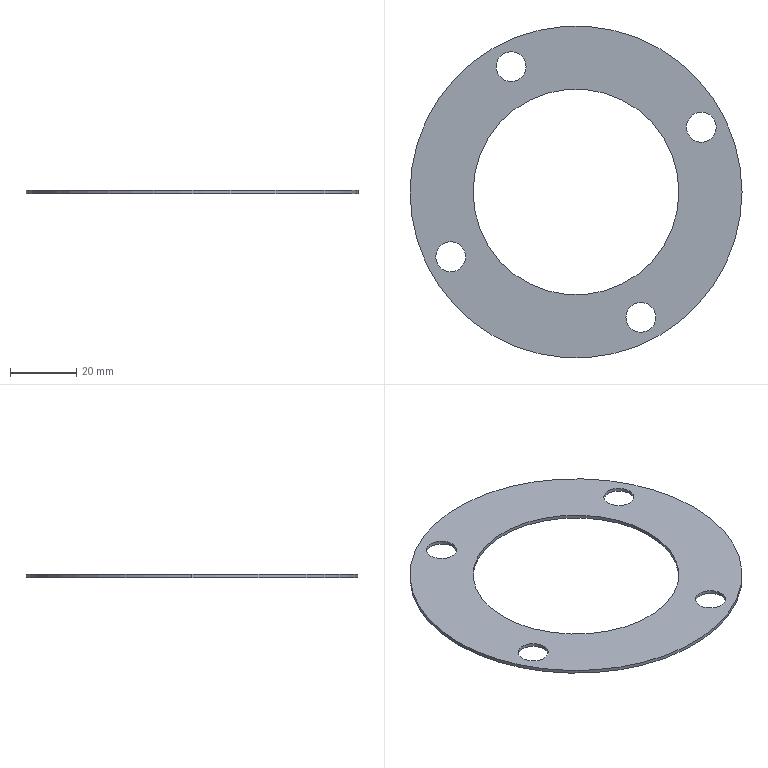Part | SolidWorks | features BaseBody 1 | 1 solid | 14 faces | box 100 x 100 x 1 mm | volume 4580 mm3 | cylinder 12 | plane 2 | commonest cylinder face diameters 9 x8 62 x2 100 x2
STEP:
#1=CARTESIAN_POINT('',(41.434,-38.434,0.));
#2=VERTEX_POINT('',#1);
#3=CARTESIAN_POINT('',(50.434,-38.434,0.));
#4=VERTEX_POINT('',#3);
#5=CARTESIAN_POINT('',(45.934,-38.434,0.));
#6=DIRECTION('',(0.,0.,1.));
#7=DIRECTION('',(1.,0.,0.));
#8=AXIS2_PLACEMENT_3D('',#5,#6,#7);
#9=CIRCLE('',#8,4.5);
#10=EDGE_CURVE('',#2,#4,#9,.T.);
#11=ORIENTED_EDGE('',*,*,#10,.F.);
#12=CARTESIAN_POINT('',(41.434,-38.434,1.));
#13=VERTEX_POINT('',#12);
#14=CARTESIAN_POINT('',(41.434,-38.434,0.));
#15=DIRECTION('',(0.,0.,1.));
#16=VECTOR('',#15,1000.);
#17=LINE('',#14,#16);
#18=EDGE_CURVE('',#2,#13,#17,.T.);
#19=ORIENTED_EDGE('',*,*,#18,.T.);
#20=CARTESIAN_POINT('',(50.434,-38.434,1.));
#21=VERTEX_POINT('',#20);
#22=CARTESIAN_POINT('',(45.934,-38.434,1.));
#23=DIRECTION('',(0.,0.,-1.));
#24=DIRECTION('',(1.,0.,0.));
#25=AXIS2_PLACEMENT_3D('',#22,#23,#24);
#26=CIRCLE('',#25,4.5);
#27=EDGE_CURVE('',#21,#13,#26,.T.);
#28=ORIENTED_EDGE('',*,*,#27,.F.);
#29=CARTESIAN_POINT('',(50.434,-38.434,0.));
#30=DIRECTION('',(0.,0.,1.));
#31=VECTOR('',#30,1000.);
#32=LINE('',#29,#31);
#33=EDGE_CURVE('',#4,#21,#32,.T.);
#34=ORIENTED_EDGE('',*,*,#33,.F.);
#35=EDGE_LOOP('',(#11,#19,#28,#34));
#36=FACE_OUTER_BOUND('',#35,.T.);
#37=CARTESIAN_POINT('',(45.934,-38.434,0.));
#38=DIRECTION('',(0.,0.,1.));
#39=DIRECTION('',(1.,0.,0.));
#40=AXIS2_PLACEMENT_3D('',#37,#38,#39);
#41=CYLINDRICAL_SURFACE('',#40,4.5);
#42=ADVANCED_FACE('',(#36),#41,.F.);
#43=CARTESIAN_POINT('',(59.662,18.839,0.));
#44=VERTEX_POINT('',#43);
#45=CARTESIAN_POINT('',(68.662,18.839,0.));
#46=VERTEX_POINT('',#45);
#47=CARTESIAN_POINT('',(64.162,18.839,0.));
#48=DIRECTION('',(0.,0.,1.));
#49=DIRECTION('',(1.,0.,0.));
#50=AXIS2_PLACEMENT_3D('',#47,#48,#49);
#51=CIRCLE('',#50,4.5);
#52=EDGE_CURVE('',#44,#46,#51,.T.);
#53=ORIENTED_EDGE('',*,*,#52,.F.);
#54=CARTESIAN_POINT('',(59.662,18.839,1.));
#55=VERTEX_POINT('',#54);
#56=CARTESIAN_POINT('',(59.662,18.839,0.));
#57=DIRECTION('',(0.,0.,1.));
#58=VECTOR('',#57,1000.);
#59=LINE('',#56,#58);
#60=EDGE_CURVE('',#44,#55,#59,.T.);
#61=ORIENTED_EDGE('',*,*,#60,.T.);
#62=CARTESIAN_POINT('',(68.662,18.839,1.));
#63=VERTEX_POINT('',#62);
#64=CARTESIAN_POINT('',(64.162,18.839,1.));
#65=DIRECTION('',(0.,0.,-1.));
#66=DIRECTION('',(1.,0.,0.));
#67=AXIS2_PLACEMENT_3D('',#64,#65,#66);
#68=CIRCLE('',#67,4.5);
#69=EDGE_CURVE('',#63,#55,#68,.T.);
#70=ORIENTED_EDGE('',*,*,#69,.F.);
#71=CARTESIAN_POINT('',(68.662,18.839,0.));
#72=DIRECTION('',(0.,0.,1.));
#73=VECTOR('',#72,1000.);
#74=LINE('',#71,#73);
#75=EDGE_CURVE('',#46,#63,#74,.T.);
#76=ORIENTED_EDGE('',*,*,#75,.F.);
#77=EDGE_LOOP('',(#53,#61,#70,#76));
#78=FACE_OUTER_BOUND('',#77,.T.);
#79=CARTESIAN_POINT('',(64.162,18.839,0.));
#80=DIRECTION('',(0.,0.,1.));
#81=DIRECTION('',(1.,0.,0.));
#82=AXIS2_PLACEMENT_3D('',#79,#80,#81);
#83=CYLINDRICAL_SURFACE('',#82,4.5);
#84=ADVANCED_FACE('',(#78),#83,.F.);
#85=CARTESIAN_POINT('',(2.389,37.067,0.));
#86=VERTEX_POINT('',#85);
#87=CARTESIAN_POINT('',(11.389,37.067,0.));
#88=VERTEX_POINT('',#87);
#89=CARTESIAN_POINT('',(6.889,37.067,0.));
#90=DIRECTION('',(0.,0.,1.));
#91=DIRECTION('',(1.,0.,0.));
#92=AXIS2_PLACEMENT_3D('',#89,#90,#91);
#93=CIRCLE('',#92,4.5);
#94=EDGE_CURVE('',#86,#88,#93,.T.);
#95=ORIENTED_EDGE('',*,*,#94,.F.);
#96=CARTESIAN_POINT('',(2.389,37.067,1.));
#97=VERTEX_POINT('',#96);
#98=CARTESIAN_POINT('',(2.389,37.067,0.));
#99=DIRECTION('',(0.,0.,1.));
#100=VECTOR('',#99,1000.);
#101=LINE('',#98,#100);
#102=EDGE_CURVE('',#86,#97,#101,.T.);
#103=ORIENTED_EDGE('',*,*,#102,.T.);
#104=CARTESIAN_POINT('',(11.389,37.067,1.));
#105=VERTEX_POINT('',#104);
#106=CARTESIAN_POINT('',(6.889,37.067,1.));
#107=DIRECTION('',(0.,0.,-1.));
#108=DIRECTION('',(1.,0.,0.));
#109=AXIS2_PLACEMENT_3D('',#106,#107,#108);
#110=CIRCLE('',#109,4.5);
#111=EDGE_CURVE('',#105,#97,#110,.T.);
#112=ORIENTED_EDGE('',*,*,#111,.F.);
#113=CARTESIAN_POINT('',(11.389,37.067,0.));
#114=DIRECTION('',(0.,0.,1.));
#115=VECTOR('',#114,1000.);
#116=LINE('',#113,#115);
#117=EDGE_CURVE('',#88,#105,#116,.T.);
#118=ORIENTED_EDGE('',*,*,#117,.F.);
#119=EDGE_LOOP('',(#95,#103,#112,#118));
#120=FACE_OUTER_BOUND('',#119,.T.);
#121=CARTESIAN_POINT('',(6.889,37.067,0.));
#122=DIRECTION('',(0.,0.,1.));
#123=DIRECTION('',(1.,0.,0.));
#124=AXIS2_PLACEMENT_3D('',#121,#122,#123);
#125=CYLINDRICAL_SURFACE('',#124,4.5);
#126=ADVANCED_FACE('',(#120),#125,.F.);
#127=CARTESIAN_POINT('',(-15.839,-20.206,0.));
#128=VERTEX_POINT('',#127);
#129=CARTESIAN_POINT('',(-6.839,-20.206,0.));
#130=VERTEX_POINT('',#129);
#131=CARTESIAN_POINT('',(-11.339,-20.206,0.));
#132=DIRECTION('',(0.,0.,1.));
#133=DIRECTION('',(1.,0.,0.));
#134=AXIS2_PLACEMENT_3D('',#131,#132,#133);
#135=CIRCLE('',#134,4.5);
#136=EDGE_CURVE('',#128,#130,#135,.T.);
#137=ORIENTED_EDGE('',*,*,#136,.F.);
#138=CARTESIAN_POINT('',(-15.839,-20.206,1.));
#139=VERTEX_POINT('',#138);
#140=CARTESIAN_POINT('',(-15.839,-20.206,0.));
#141=DIRECTION('',(0.,0.,1.));
#142=VECTOR('',#141,1000.);
#143=LINE('',#140,#142);
#144=EDGE_CURVE('',#128,#139,#143,.T.);
#145=ORIENTED_EDGE('',*,*,#144,.T.);
#146=CARTESIAN_POINT('',(-6.839,-20.206,1.));
#147=VERTEX_POINT('',#146);
#148=CARTESIAN_POINT('',(-11.339,-20.206,1.));
#149=DIRECTION('',(0.,0.,-1.));
#150=DIRECTION('',(1.,0.,0.));
#151=AXIS2_PLACEMENT_3D('',#148,#149,#150);
#152=CIRCLE('',#151,4.5);
#153=EDGE_CURVE('',#147,#139,#152,.T.);
#154=ORIENTED_EDGE('',*,*,#153,.F.);
#155=CARTESIAN_POINT('',(-6.839,-20.206,0.));
#156=DIRECTION('',(0.,0.,1.));
#157=VECTOR('',#156,1000.);
#158=LINE('',#155,#157);
#159=EDGE_CURVE('',#130,#147,#158,.T.);
#160=ORIENTED_EDGE('',*,*,#159,.F.);
#161=EDGE_LOOP('',(#137,#145,#154,#160));
#162=FACE_OUTER_BOUND('',#161,.T.);
#163=CARTESIAN_POINT('',(-11.339,-20.206,0.));
#164=DIRECTION('',(0.,0.,1.));
#165=DIRECTION('',(1.,0.,0.));
#166=AXIS2_PLACEMENT_3D('',#163,#164,#165);
#167=CYLINDRICAL_SURFACE('',#166,4.5);
#168=ADVANCED_FACE('',(#162),#167,.F.);
#169=CARTESIAN_POINT('',(-4.588,-0.6833,0.));
#170=VERTEX_POINT('',#169);
#171=CARTESIAN_POINT('',(57.412,-0.6833,0.));
#172=VERTEX_POINT('',#171);
#173=CARTESIAN_POINT('',(26.412,-0.6833,0.));
#174=DIRECTION('',(0.,0.,1.));
#175=DIRECTION('',(1.,0.,0.));
#176=AXIS2_PLACEMENT_3D('',#173,#174,#175);
#177=CIRCLE('',#176,31.);
#178=EDGE_CURVE('',#170,#172,#177,.T.);
#179=ORIENTED_EDGE('',*,*,#178,.F.);
#180=CARTESIAN_POINT('',(-4.588,-0.6833,1.));
#181=VERTEX_POINT('',#180);
#182=CARTESIAN_POINT('',(-4.588,-0.6833,0.));
#183=DIRECTION('',(0.,0.,1.));
#184=VECTOR('',#183,1000.);
#185=LINE('',#182,#184);
#186=EDGE_CURVE('',#170,#181,#185,.T.);
#187=ORIENTED_EDGE('',*,*,#186,.T.);
#188=CARTESIAN_POINT('',(57.412,-0.6833,1.));
#189=VERTEX_POINT('',#188);
#190=CARTESIAN_POINT('',(26.412,-0.6833,1.));
#191=DIRECTION('',(0.,0.,-1.));
#192=DIRECTION('',(1.,0.,0.));
#193=AXIS2_PLACEMENT_3D('',#190,#191,#192);
#194=CIRCLE('',#193,31.);
#195=EDGE_CURVE('',#189,#181,#194,.T.);
#196=ORIENTED_EDGE('',*,*,#195,.F.);
#197=CARTESIAN_POINT('',(57.412,-0.6833,0.));
#198=DIRECTION('',(0.,0.,1.));
#199=VECTOR('',#198,1000.);
#200=LINE('',#197,#199);
#201=EDGE_CURVE('',#172,#189,#200,.T.);
#202=ORIENTED_EDGE('',*,*,#201,.F.);
#203=EDGE_LOOP('',(#179,#187,#196,#202));
#204=FACE_OUTER_BOUND('',#203,.T.);
#205=CARTESIAN_POINT('',(26.412,-0.6833,0.));
#206=DIRECTION('',(0.,0.,1.));
#207=DIRECTION('',(1.,0.,0.));
#208=AXIS2_PLACEMENT_3D('',#205,#206,#207);
#209=CYLINDRICAL_SURFACE('',#208,31.);
#210=ADVANCED_FACE('',(#204),#209,.F.);
#211=CARTESIAN_POINT('',(76.412,-0.6833,0.));
#212=VERTEX_POINT('',#211);
#213=CARTESIAN_POINT('',(-23.588,-0.6833,0.));
#214=VERTEX_POINT('',#213);
#215=CARTESIAN_POINT('',(26.412,-0.6833,0.));
#216=DIRECTION('',(0.,0.,1.));
#217=DIRECTION('',(1.,0.,0.));
#218=AXIS2_PLACEMENT_3D('',#215,#216,#217);
#219=CIRCLE('',#218,50.);
#220=EDGE_CURVE('',#212,#214,#219,.T.);
#221=ORIENTED_EDGE('',*,*,#220,.T.);
#222=CARTESIAN_POINT('',(-23.588,-0.6833,1.));
#223=VERTEX_POINT('',#222);
#224=CARTESIAN_POINT('',(-23.588,-0.6833,0.));
#225=DIRECTION('',(0.,0.,1.));
#226=VECTOR('',#225,1000.);
#227=LINE('',#224,#226);
#228=EDGE_CURVE('',#214,#223,#227,.T.);
#229=ORIENTED_EDGE('',*,*,#228,.T.);
#230=CARTESIAN_POINT('',(76.412,-0.6833,1.));
#231=VERTEX_POINT('',#230);
#232=CARTESIAN_POINT('',(26.412,-0.6833,1.));
#233=DIRECTION('',(0.,0.,1.));
#234=DIRECTION('',(1.,0.,0.));
#235=AXIS2_PLACEMENT_3D('',#232,#233,#234);
#236=CIRCLE('',#235,50.);
#237=EDGE_CURVE('',#231,#223,#236,.T.);
#238=ORIENTED_EDGE('',*,*,#237,.F.);
#239=CARTESIAN_POINT('',(76.412,-0.6833,0.));
#240=DIRECTION('',(0.,0.,1.));
#241=VECTOR('',#240,1000.);
#242=LINE('',#239,#241);
#243=EDGE_CURVE('',#212,#231,#242,.T.);
#244=ORIENTED_EDGE('',*,*,#243,.F.);
#245=EDGE_LOOP('',(#221,#229,#238,#244));
#246=FACE_OUTER_BOUND('',#245,.T.);
#247=CARTESIAN_POINT('',(26.412,-0.6833,0.));
#248=DIRECTION('',(0.,0.,1.));
#249=DIRECTION('',(1.,0.,0.));
#250=AXIS2_PLACEMENT_3D('',#247,#248,#249);
#251=CYLINDRICAL_SURFACE('',#250,50.);
#252=ADVANCED_FACE('',(#246),#251,.T.);
#253=ORIENTED_EDGE('',*,*,#27,.T.);
#254=CARTESIAN_POINT('',(45.934,-38.434,1.));
#255=DIRECTION('',(0.,0.,-1.));
#256=DIRECTION('',(1.,0.,0.));
#257=AXIS2_PLACEMENT_3D('',#254,#255,#256);
#258=CIRCLE('',#257,4.5);
#259=EDGE_CURVE('',#13,#21,#258,.T.);
#260=ORIENTED_EDGE('',*,*,#259,.T.);
#261=EDGE_LOOP('',(#253,#260));
#262=FACE_BOUND('',#261,.T.);
#263=ORIENTED_EDGE('',*,*,#69,.T.);
#264=CARTESIAN_POINT('',(64.162,18.839,1.));
#265=DIRECTION('',(0.,0.,-1.));
#266=DIRECTION('',(1.,0.,0.));
#267=AXIS2_PLACEMENT_3D('',#264,#265,#266);
#268=CIRCLE('',#267,4.5);
#269=EDGE_CURVE('',#55,#63,#268,.T.);
#270=ORIENTED_EDGE('',*,*,#269,.T.);
#271=EDGE_LOOP('',(#263,#270));
#272=FACE_BOUND('',#271,.T.);
#273=ORIENTED_EDGE('',*,*,#111,.T.);
#274=CARTESIAN_POINT('',(6.889,37.067,1.));
#275=DIRECTION('',(0.,0.,-1.));
#276=DIRECTION('',(1.,0.,0.));
#277=AXIS2_PLACEMENT_3D('',#274,#275,#276);
#278=CIRCLE('',#277,4.5);
#279=EDGE_CURVE('',#97,#105,#278,.T.);
#280=ORIENTED_EDGE('',*,*,#279,.T.);
#281=EDGE_LOOP('',(#273,#280));
#282=FACE_BOUND('',#281,.T.);
#283=ORIENTED_EDGE('',*,*,#153,.T.);
#284=CARTESIAN_POINT('',(-11.339,-20.206,1.));
#285=DIRECTION('',(0.,0.,-1.));
#286=DIRECTION('',(1.,0.,0.));
#287=AXIS2_PLACEMENT_3D('',#284,#285,#286);
#288=CIRCLE('',#287,4.5);
#289=EDGE_CURVE('',#139,#147,#288,.T.);
#290=ORIENTED_EDGE('',*,*,#289,.T.);
#291=EDGE_LOOP('',(#283,#290));
#292=FACE_BOUND('',#291,.T.);
#293=ORIENTED_EDGE('',*,*,#195,.T.);
#294=CARTESIAN_POINT('',(26.412,-0.6833,1.));
#295=DIRECTION('',(0.,0.,-1.));
#296=DIRECTION('',(1.,0.,0.));
#297=AXIS2_PLACEMENT_3D('',#294,#295,#296);
#298=CIRCLE('',#297,31.);
#299=EDGE_CURVE('',#181,#189,#298,.T.);
#300=ORIENTED_EDGE('',*,*,#299,.T.);
#301=EDGE_LOOP('',(#293,#300));
#302=FACE_BOUND('',#301,.T.);
#303=ORIENTED_EDGE('',*,*,#237,.T.);
#304=CARTESIAN_POINT('',(26.412,-0.6833,1.));
#305=DIRECTION('',(0.,0.,1.));
#306=DIRECTION('',(1.,0.,0.));
#307=AXIS2_PLACEMENT_3D('',#304,#305,#306);
#308=CIRCLE('',#307,50.);
#309=EDGE_CURVE('',#223,#231,#308,.T.);
#310=ORIENTED_EDGE('',*,*,#309,.T.);
#311=EDGE_LOOP('',(#303,#310));
#312=FACE_OUTER_BOUND('',#311,.T.);
#313=CARTESIAN_POINT('',(26.412,-0.6833,1.));
#314=DIRECTION('',(0.,0.,1.));
#315=DIRECTION('',(1.,0.,0.));
#316=AXIS2_PLACEMENT_3D('',#313,#314,#315);
#317=PLANE('',#316);
#318=ADVANCED_FACE('',(#262,#272,#282,#292,#302,#312),#317,.T.);
#319=ORIENTED_EDGE('',*,*,#18,.F.);
#320=CARTESIAN_POINT('',(45.934,-38.434,0.));
#321=DIRECTION('',(0.,0.,1.));
#322=DIRECTION('',(1.,0.,0.));
#323=AXIS2_PLACEMENT_3D('',#320,#321,#322);
#324=CIRCLE('',#323,4.5);
#325=EDGE_CURVE('',#4,#2,#324,.T.);
#326=ORIENTED_EDGE('',*,*,#325,.F.);
#327=ORIENTED_EDGE('',*,*,#33,.T.);
#328=ORIENTED_EDGE('',*,*,#259,.F.);
#329=EDGE_LOOP('',(#319,#326,#327,#328));
#330=FACE_OUTER_BOUND('',#329,.T.);
#331=CARTESIAN_POINT('',(45.934,-38.434,0.));
#332=DIRECTION('',(0.,0.,1.));
#333=DIRECTION('',(1.,0.,0.));
#334=AXIS2_PLACEMENT_3D('',#331,#332,#333);
#335=CYLINDRICAL_SURFACE('',#334,4.5);
#336=ADVANCED_FACE('',(#330),#335,.F.);
#337=ORIENTED_EDGE('',*,*,#60,.F.);
#338=CARTESIAN_POINT('',(64.162,18.839,0.));
#339=DIRECTION('',(0.,0.,1.));
#340=DIRECTION('',(1.,0.,0.));
#341=AXIS2_PLACEMENT_3D('',#338,#339,#340);
#342=CIRCLE('',#341,4.5);
#343=EDGE_CURVE('',#46,#44,#342,.T.);
#344=ORIENTED_EDGE('',*,*,#343,.F.);
#345=ORIENTED_EDGE('',*,*,#75,.T.);
#346=ORIENTED_EDGE('',*,*,#269,.F.);
#347=EDGE_LOOP('',(#337,#344,#345,#346));
#348=FACE_OUTER_BOUND('',#347,.T.);
#349=CARTESIAN_POINT('',(64.162,18.839,0.));
#350=DIRECTION('',(0.,0.,1.));
#351=DIRECTION('',(1.,0.,0.));
#352=AXIS2_PLACEMENT_3D('',#349,#350,#351);
#353=CYLINDRICAL_SURFACE('',#352,4.5);
#354=ADVANCED_FACE('',(#348),#353,.F.);
#355=ORIENTED_EDGE('',*,*,#102,.F.);
#356=CARTESIAN_POINT('',(6.889,37.067,0.));
#357=DIRECTION('',(0.,0.,1.));
#358=DIRECTION('',(1.,0.,0.));
#359=AXIS2_PLACEMENT_3D('',#356,#357,#358);
#360=CIRCLE('',#359,4.5);
#361=EDGE_CURVE('',#88,#86,#360,.T.);
#362=ORIENTED_EDGE('',*,*,#361,.F.);
#363=ORIENTED_EDGE('',*,*,#117,.T.);
#364=ORIENTED_EDGE('',*,*,#279,.F.);
#365=EDGE_LOOP('',(#355,#362,#363,#364));
#366=FACE_OUTER_BOUND('',#365,.T.);
#367=CARTESIAN_POINT('',(6.889,37.067,0.));
#368=DIRECTION('',(0.,0.,1.));
#369=DIRECTION('',(1.,0.,0.));
#370=AXIS2_PLACEMENT_3D('',#367,#368,#369);
#371=CYLINDRICAL_SURFACE('',#370,4.5);
#372=ADVANCED_FACE('',(#366),#371,.F.);
#373=ORIENTED_EDGE('',*,*,#144,.F.);
#374=CARTESIAN_POINT('',(-11.339,-20.206,0.));
#375=DIRECTION('',(0.,0.,1.));
#376=DIRECTION('',(1.,0.,0.));
#377=AXIS2_PLACEMENT_3D('',#374,#375,#376);
#378=CIRCLE('',#377,4.5);
#379=EDGE_CURVE('',#130,#128,#378,.T.);
#380=ORIENTED_EDGE('',*,*,#379,.F.);
#381=ORIENTED_EDGE('',*,*,#159,.T.);
#382=ORIENTED_EDGE('',*,*,#289,.F.);
#383=EDGE_LOOP('',(#373,#380,#381,#382));
#384=FACE_OUTER_BOUND('',#383,.T.);
#385=CARTESIAN_POINT('',(-11.339,-20.206,0.));
#386=DIRECTION('',(0.,0.,1.));
#387=DIRECTION('',(1.,0.,0.));
#388=AXIS2_PLACEMENT_3D('',#385,#386,#387);
#389=CYLINDRICAL_SURFACE('',#388,4.5);
#390=ADVANCED_FACE('',(#384),#389,.F.);
#391=ORIENTED_EDGE('',*,*,#186,.F.);
#392=CARTESIAN_POINT('',(26.412,-0.6833,0.));
#393=DIRECTION('',(0.,0.,1.));
#394=DIRECTION('',(1.,0.,0.));
#395=AXIS2_PLACEMENT_3D('',#392,#393,#394);
#396=CIRCLE('',#395,31.);
#397=EDGE_CURVE('',#172,#170,#396,.T.);
#398=ORIENTED_EDGE('',*,*,#397,.F.);
#399=ORIENTED_EDGE('',*,*,#201,.T.);
#400=ORIENTED_EDGE('',*,*,#299,.F.);
#401=EDGE_LOOP('',(#391,#398,#399,#400));
#402=FACE_OUTER_BOUND('',#401,.T.);
#403=CARTESIAN_POINT('',(26.412,-0.6833,0.));
#404=DIRECTION('',(0.,0.,1.));
#405=DIRECTION('',(1.,0.,0.));
#406=AXIS2_PLACEMENT_3D('',#403,#404,#405);
#407=CYLINDRICAL_SURFACE('',#406,31.);
#408=ADVANCED_FACE('',(#402),#407,.F.);
#409=ORIENTED_EDGE('',*,*,#228,.F.);
#410=CARTESIAN_POINT('',(26.412,-0.6833,0.));
#411=DIRECTION('',(0.,0.,1.));
#412=DIRECTION('',(1.,0.,0.));
#413=AXIS2_PLACEMENT_3D('',#410,#411,#412);
#414=CIRCLE('',#413,50.);
#415=EDGE_CURVE('',#214,#212,#414,.T.);
#416=ORIENTED_EDGE('',*,*,#415,.T.);
#417=ORIENTED_EDGE('',*,*,#243,.T.);
#418=ORIENTED_EDGE('',*,*,#309,.F.);
#419=EDGE_LOOP('',(#409,#416,#417,#418));
#420=FACE_OUTER_BOUND('',#419,.T.);
#421=CARTESIAN_POINT('',(26.412,-0.6833,0.));
#422=DIRECTION('',(0.,0.,1.));
#423=DIRECTION('',(1.,0.,0.));
#424=AXIS2_PLACEMENT_3D('',#421,#422,#423);
#425=CYLINDRICAL_SURFACE('',#424,50.);
#426=ADVANCED_FACE('',(#420),#425,.T.);
#427=ORIENTED_EDGE('',*,*,#325,.T.);
#428=ORIENTED_EDGE('',*,*,#10,.T.);
#429=EDGE_LOOP('',(#427,#428));
#430=FACE_BOUND('',#429,.T.);
#431=ORIENTED_EDGE('',*,*,#343,.T.);
#432=ORIENTED_EDGE('',*,*,#52,.T.);
#433=EDGE_LOOP('',(#431,#432));
#434=FACE_BOUND('',#433,.T.);
#435=ORIENTED_EDGE('',*,*,#361,.T.);
#436=ORIENTED_EDGE('',*,*,#94,.T.);
#437=EDGE_LOOP('',(#435,#436));
#438=FACE_BOUND('',#437,.T.);
#439=ORIENTED_EDGE('',*,*,#379,.T.);
#440=ORIENTED_EDGE('',*,*,#136,.T.);
#441=EDGE_LOOP('',(#439,#440));
#442=FACE_BOUND('',#441,.T.);
#443=ORIENTED_EDGE('',*,*,#397,.T.);
#444=ORIENTED_EDGE('',*,*,#178,.T.);
#445=EDGE_LOOP('',(#443,#444));
#446=FACE_BOUND('',#445,.T.);
#447=ORIENTED_EDGE('',*,*,#220,.F.);
#448=ORIENTED_EDGE('',*,*,#415,.F.);
#449=EDGE_LOOP('',(#447,#448));
#450=FACE_OUTER_BOUND('',#449,.T.);
#451=CARTESIAN_POINT('',(26.412,-0.6833,0.));
#452=DIRECTION('',(0.,0.,1.));
#453=DIRECTION('',(1.,0.,0.));
#454=AXIS2_PLACEMENT_3D('',#451,#452,#453);
#455=PLANE('',#454);
#456=ADVANCED_FACE('',(#430,#434,#438,#442,#446,#450),#455,.F.);
#457=CLOSED_SHELL('',(#42,#84,#126,#168,#210,#252,#318,#336,#354,#372,#390,#408,#426,#456));
#458=MANIFOLD_SOLID_BREP('',#457);
#459=CARTESIAN_POINT('',(0.,0.,0.));
#460=DIRECTION('',(0.,0.,1.));
#461=DIRECTION('',(1.,0.,0.));
#462=AXIS2_PLACEMENT_3D('',#459,#460,#461);
#463=(LENGTH_UNIT()NAMED_UNIT(*)SI_UNIT(.MILLI.,.METRE.));
#464=UNCERTAINTY_MEASURE_WITH_UNIT(LENGTH_MEASURE(0.00001),#463,'','');
#465=(NAMED_UNIT(*)PLANE_ANGLE_UNIT()SI_UNIT($,.RADIAN.));
#466=(NAMED_UNIT(*)SI_UNIT($,.STERADIAN.)SOLID_ANGLE_UNIT());
#467=(GEOMETRIC_REPRESENTATION_CONTEXT(3)GLOBAL_UNCERTAINTY_ASSIGNED_CONTEXT((#464))GLOBAL_UNIT_ASSIGNED_CONTEXT((#463,#465,#466))REPRESENTATION_CONTEXT('',''));
#468=ADVANCED_BREP_SHAPE_REPRESENTATION('',(#458,#462),#467);